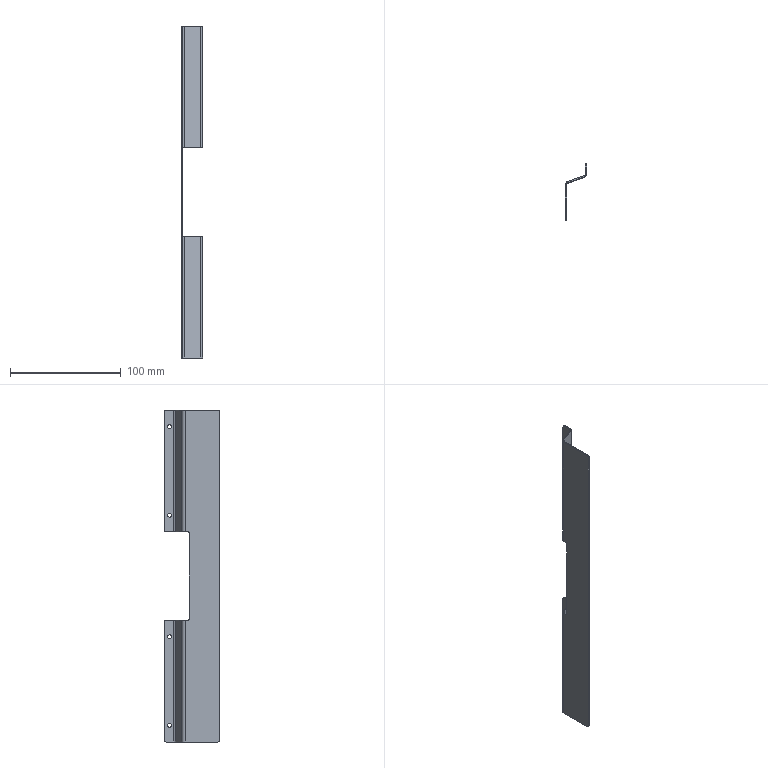Part | SolidWorks | features BaseBody 1 | 1 solid | 42 faces | box 19 x 50.551 x 300 mm | volume 15860 mm3 | cylinder 24 | plane 18 | commonest cylinder face diameters 4 x12 3.5 x8 6 x4
STEP:
#1=CARTESIAN_POINT('',(0.,6.,-53.25));
#2=VERTEX_POINT('',#1);
#3=CARTESIAN_POINT('',(0.,6.,-56.75));
#4=VERTEX_POINT('',#3);
#5=CARTESIAN_POINT('',(0.,6.,-55.));
#6=DIRECTION('',(1.,0.,0.));
#7=DIRECTION('',(0.,1.,0.));
#8=AXIS2_PLACEMENT_3D('',#5,#6,#7);
#9=CIRCLE('',#8,1.75);
#10=EDGE_CURVE('',#2,#4,#9,.T.);
#11=ORIENTED_EDGE('',*,*,#10,.T.);
#12=CARTESIAN_POINT('',(-1.,6.,-56.75));
#13=VERTEX_POINT('',#12);
#14=CARTESIAN_POINT('',(-1.,6.,-56.75));
#15=DIRECTION('',(-1.,0.,0.));
#16=VECTOR('',#15,1000.);
#17=LINE('',#14,#16);
#18=EDGE_CURVE('',#4,#13,#17,.T.);
#19=ORIENTED_EDGE('',*,*,#18,.T.);
#20=CARTESIAN_POINT('',(-1.,6.,-53.25));
#21=VERTEX_POINT('',#20);
#22=CARTESIAN_POINT('',(-1.,6.,-55.));
#23=DIRECTION('',(-1.,0.,0.));
#24=DIRECTION('',(0.,0.,1.));
#25=AXIS2_PLACEMENT_3D('',#22,#23,#24);
#26=CIRCLE('',#25,1.75);
#27=EDGE_CURVE('',#13,#21,#26,.T.);
#28=ORIENTED_EDGE('',*,*,#27,.T.);
#29=CARTESIAN_POINT('',(-1.,6.,-53.25));
#30=DIRECTION('',(-1.,0.,0.));
#31=VECTOR('',#30,1000.);
#32=LINE('',#29,#31);
#33=EDGE_CURVE('',#2,#21,#32,.T.);
#34=ORIENTED_EDGE('',*,*,#33,.F.);
#35=EDGE_LOOP('',(#11,#19,#28,#34));
#36=FACE_OUTER_BOUND('',#35,.T.);
#37=CARTESIAN_POINT('',(-1.,6.,-55.));
#38=DIRECTION('',(-1.,0.,0.));
#39=DIRECTION('',(0.,0.,1.));
#40=AXIS2_PLACEMENT_3D('',#37,#38,#39);
#41=CYLINDRICAL_SURFACE('',#40,1.75);
#42=ADVANCED_FACE('',(#36),#41,.F.);
#43=CARTESIAN_POINT('',(0.,6.,56.75));
#44=VERTEX_POINT('',#43);
#45=CARTESIAN_POINT('',(0.,6.,53.25));
#46=VERTEX_POINT('',#45);
#47=CARTESIAN_POINT('',(0.,6.,55.));
#48=DIRECTION('',(1.,0.,0.));
#49=DIRECTION('',(0.,1.,0.));
#50=AXIS2_PLACEMENT_3D('',#47,#48,#49);
#51=CIRCLE('',#50,1.75);
#52=EDGE_CURVE('',#44,#46,#51,.T.);
#53=ORIENTED_EDGE('',*,*,#52,.T.);
#54=CARTESIAN_POINT('',(-1.,6.,53.25));
#55=VERTEX_POINT('',#54);
#56=CARTESIAN_POINT('',(-1.,6.,53.25));
#57=DIRECTION('',(-1.,0.,0.));
#58=VECTOR('',#57,1000.);
#59=LINE('',#56,#58);
#60=EDGE_CURVE('',#46,#55,#59,.T.);
#61=ORIENTED_EDGE('',*,*,#60,.T.);
#62=CARTESIAN_POINT('',(-1.,6.,56.75));
#63=VERTEX_POINT('',#62);
#64=CARTESIAN_POINT('',(-1.,6.,55.));
#65=DIRECTION('',(-1.,0.,0.));
#66=DIRECTION('',(0.,0.,1.));
#67=AXIS2_PLACEMENT_3D('',#64,#65,#66);
#68=CIRCLE('',#67,1.75);
#69=EDGE_CURVE('',#55,#63,#68,.T.);
#70=ORIENTED_EDGE('',*,*,#69,.T.);
#71=CARTESIAN_POINT('',(-1.,6.,56.75));
#72=DIRECTION('',(-1.,0.,0.));
#73=VECTOR('',#72,1000.);
#74=LINE('',#71,#73);
#75=EDGE_CURVE('',#44,#63,#74,.T.);
#76=ORIENTED_EDGE('',*,*,#75,.F.);
#77=EDGE_LOOP('',(#53,#61,#70,#76));
#78=FACE_OUTER_BOUND('',#77,.T.);
#79=CARTESIAN_POINT('',(-1.,6.,55.));
#80=DIRECTION('',(-1.,0.,0.));
#81=DIRECTION('',(0.,0.,1.));
#82=AXIS2_PLACEMENT_3D('',#79,#80,#81);
#83=CYLINDRICAL_SURFACE('',#82,1.75);
#84=ADVANCED_FACE('',(#78),#83,.F.);
#85=CARTESIAN_POINT('',(0.,6.,-133.25));
#86=VERTEX_POINT('',#85);
#87=CARTESIAN_POINT('',(0.,6.,-136.75));
#88=VERTEX_POINT('',#87);
#89=CARTESIAN_POINT('',(0.,6.,-135.));
#90=DIRECTION('',(1.,0.,0.));
#91=DIRECTION('',(0.,1.,0.));
#92=AXIS2_PLACEMENT_3D('',#89,#90,#91);
#93=CIRCLE('',#92,1.75);
#94=EDGE_CURVE('',#86,#88,#93,.T.);
#95=ORIENTED_EDGE('',*,*,#94,.T.);
#96=CARTESIAN_POINT('',(-1.,6.,-136.75));
#97=VERTEX_POINT('',#96);
#98=CARTESIAN_POINT('',(-1.,6.,-136.75));
#99=DIRECTION('',(-1.,0.,0.));
#100=VECTOR('',#99,1000.);
#101=LINE('',#98,#100);
#102=EDGE_CURVE('',#88,#97,#101,.T.);
#103=ORIENTED_EDGE('',*,*,#102,.T.);
#104=CARTESIAN_POINT('',(-1.,6.,-133.25));
#105=VERTEX_POINT('',#104);
#106=CARTESIAN_POINT('',(-1.,6.,-135.));
#107=DIRECTION('',(-1.,0.,0.));
#108=DIRECTION('',(0.,0.,1.));
#109=AXIS2_PLACEMENT_3D('',#106,#107,#108);
#110=CIRCLE('',#109,1.75);
#111=EDGE_CURVE('',#97,#105,#110,.T.);
#112=ORIENTED_EDGE('',*,*,#111,.T.);
#113=CARTESIAN_POINT('',(-1.,6.,-133.25));
#114=DIRECTION('',(-1.,0.,0.));
#115=VECTOR('',#114,1000.);
#116=LINE('',#113,#115);
#117=EDGE_CURVE('',#86,#105,#116,.T.);
#118=ORIENTED_EDGE('',*,*,#117,.F.);
#119=EDGE_LOOP('',(#95,#103,#112,#118));
#120=FACE_OUTER_BOUND('',#119,.T.);
#121=CARTESIAN_POINT('',(-1.,6.,-135.));
#122=DIRECTION('',(-1.,0.,0.));
#123=DIRECTION('',(0.,0.,1.));
#124=AXIS2_PLACEMENT_3D('',#121,#122,#123);
#125=CYLINDRICAL_SURFACE('',#124,1.75);
#126=ADVANCED_FACE('',(#120),#125,.F.);
#127=CARTESIAN_POINT('',(0.,6.,136.75));
#128=VERTEX_POINT('',#127);
#129=CARTESIAN_POINT('',(0.,6.,133.25));
#130=VERTEX_POINT('',#129);
#131=CARTESIAN_POINT('',(0.,6.,135.));
#132=DIRECTION('',(1.,0.,0.));
#133=DIRECTION('',(0.,1.,0.));
#134=AXIS2_PLACEMENT_3D('',#131,#132,#133);
#135=CIRCLE('',#134,1.75);
#136=EDGE_CURVE('',#128,#130,#135,.T.);
#137=ORIENTED_EDGE('',*,*,#136,.T.);
#138=CARTESIAN_POINT('',(-1.,6.,133.25));
#139=VERTEX_POINT('',#138);
#140=CARTESIAN_POINT('',(-1.,6.,133.25));
#141=DIRECTION('',(-1.,0.,0.));
#142=VECTOR('',#141,1000.);
#143=LINE('',#140,#142);
#144=EDGE_CURVE('',#130,#139,#143,.T.);
#145=ORIENTED_EDGE('',*,*,#144,.T.);
#146=CARTESIAN_POINT('',(-1.,6.,136.75));
#147=VERTEX_POINT('',#146);
#148=CARTESIAN_POINT('',(-1.,6.,135.));
#149=DIRECTION('',(-1.,0.,0.));
#150=DIRECTION('',(0.,0.,1.));
#151=AXIS2_PLACEMENT_3D('',#148,#149,#150);
#152=CIRCLE('',#151,1.75);
#153=EDGE_CURVE('',#139,#147,#152,.T.);
#154=ORIENTED_EDGE('',*,*,#153,.T.);
#155=CARTESIAN_POINT('',(-1.,6.,136.75));
#156=DIRECTION('',(-1.,0.,0.));
#157=VECTOR('',#156,1000.);
#158=LINE('',#155,#157);
#159=EDGE_CURVE('',#128,#147,#158,.T.);
#160=ORIENTED_EDGE('',*,*,#159,.F.);
#161=EDGE_LOOP('',(#137,#145,#154,#160));
#162=FACE_OUTER_BOUND('',#161,.T.);
#163=CARTESIAN_POINT('',(-1.,6.,135.));
#164=DIRECTION('',(-1.,0.,0.));
#165=DIRECTION('',(0.,0.,1.));
#166=AXIS2_PLACEMENT_3D('',#163,#164,#165);
#167=CYLINDRICAL_SURFACE('',#166,1.75);
#168=ADVANCED_FACE('',(#162),#167,.F.);
#169=CARTESIAN_POINT('',(-1.,11.,-148.));
#170=VERTEX_POINT('',#169);
#171=CARTESIAN_POINT('',(-1.,9.,-150.));
#172=VERTEX_POINT('',#171);
#173=CARTESIAN_POINT('',(-1.,9.,-148.));
#174=DIRECTION('',(-1.,0.,0.));
#175=DIRECTION('',(0.,1.,0.));
#176=AXIS2_PLACEMENT_3D('',#173,#174,#175);
#177=CIRCLE('',#176,2.);
#178=EDGE_CURVE('',#170,#172,#177,.T.);
#179=ORIENTED_EDGE('',*,*,#178,.F.);
#180=CARTESIAN_POINT('',(0.,11.,-148.));
#181=VERTEX_POINT('',#180);
#182=CARTESIAN_POINT('',(-1.,11.,-148.));
#183=DIRECTION('',(-1.,0.,0.));
#184=VECTOR('',#183,1000.);
#185=LINE('',#182,#184);
#186=EDGE_CURVE('',#181,#170,#185,.T.);
#187=ORIENTED_EDGE('',*,*,#186,.F.);
#188=CARTESIAN_POINT('',(0.,9.,-150.));
#189=VERTEX_POINT('',#188);
#190=CARTESIAN_POINT('',(0.,9.,-148.));
#191=DIRECTION('',(1.,0.,0.));
#192=DIRECTION('',(0.,1.,0.));
#193=AXIS2_PLACEMENT_3D('',#190,#191,#192);
#194=CIRCLE('',#193,2.);
#195=EDGE_CURVE('',#189,#181,#194,.T.);
#196=ORIENTED_EDGE('',*,*,#195,.F.);
#197=CARTESIAN_POINT('',(-2.316,9.,-150.));
#198=DIRECTION('',(1.,0.,0.));
#199=VECTOR('',#198,1000.);
#200=LINE('',#197,#199);
#201=EDGE_CURVE('',#172,#189,#200,.T.);
#202=ORIENTED_EDGE('',*,*,#201,.F.);
#203=EDGE_LOOP('',(#179,#187,#196,#202));
#204=FACE_OUTER_BOUND('',#203,.T.);
#205=CARTESIAN_POINT('',(-2.316,9.,-148.));
#206=DIRECTION('',(1.,0.,0.));
#207=DIRECTION('',(0.,0.,-1.));
#208=AXIS2_PLACEMENT_3D('',#205,#206,#207);
#209=CYLINDRICAL_SURFACE('',#208,2.);
#210=ADVANCED_FACE('',(#204),#209,.T.);
#211=CARTESIAN_POINT('',(0.,11.,-42.));
#212=VERTEX_POINT('',#211);
#213=CARTESIAN_POINT('',(0.,9.,-40.));
#214=VERTEX_POINT('',#213);
#215=CARTESIAN_POINT('',(0.,9.,-42.));
#216=DIRECTION('',(1.,0.,0.));
#217=DIRECTION('',(0.,1.,0.));
#218=AXIS2_PLACEMENT_3D('',#215,#216,#217);
#219=CIRCLE('',#218,2.);
#220=EDGE_CURVE('',#212,#214,#219,.T.);
#221=ORIENTED_EDGE('',*,*,#220,.F.);
#222=CARTESIAN_POINT('',(-1.,11.,-42.));
#223=VERTEX_POINT('',#222);
#224=CARTESIAN_POINT('',(0.,11.,-42.));
#225=DIRECTION('',(1.,0.,0.));
#226=VECTOR('',#225,1000.);
#227=LINE('',#224,#226);
#228=EDGE_CURVE('',#223,#212,#227,.T.);
#229=ORIENTED_EDGE('',*,*,#228,.F.);
#230=CARTESIAN_POINT('',(-1.,9.,-40.));
#231=VERTEX_POINT('',#230);
#232=CARTESIAN_POINT('',(-1.,9.,-42.));
#233=DIRECTION('',(-1.,0.,0.));
#234=DIRECTION('',(0.,1.,0.));
#235=AXIS2_PLACEMENT_3D('',#232,#233,#234);
#236=CIRCLE('',#235,2.);
#237=EDGE_CURVE('',#231,#223,#236,.T.);
#238=ORIENTED_EDGE('',*,*,#237,.F.);
#239=CARTESIAN_POINT('',(-1.,9.,-40.));
#240=DIRECTION('',(-1.,0.,0.));
#241=VECTOR('',#240,1000.);
#242=LINE('',#239,#241);
#243=EDGE_CURVE('',#214,#231,#242,.T.);
#244=ORIENTED_EDGE('',*,*,#243,.F.);
#245=EDGE_LOOP('',(#221,#229,#238,#244));
#246=FACE_OUTER_BOUND('',#245,.T.);
#247=CARTESIAN_POINT('',(0.,9.,-42.));
#248=DIRECTION('',(1.,0.,0.));
#249=DIRECTION('',(0.,0.,-1.));
#250=AXIS2_PLACEMENT_3D('',#247,#248,#249);
#251=CYLINDRICAL_SURFACE('',#250,2.);
#252=ADVANCED_FACE('',(#246),#251,.T.);
#253=CARTESIAN_POINT('',(-18.,-10.,-40.));
#254=VERTEX_POINT('',#253);
#255=CARTESIAN_POINT('',(-18.,-12.,-38.));
#256=VERTEX_POINT('',#255);
#257=CARTESIAN_POINT('',(-18.,-10.,-38.));
#258=DIRECTION('',(-1.,0.,0.));
#259=DIRECTION('',(0.,1.,0.));
#260=AXIS2_PLACEMENT_3D('',#257,#258,#259);
#261=CIRCLE('',#260,2.);
#262=EDGE_CURVE('',#254,#256,#261,.T.);
#263=ORIENTED_EDGE('',*,*,#262,.F.);
#264=CARTESIAN_POINT('',(-19.,-10.,-40.));
#265=VERTEX_POINT('',#264);
#266=CARTESIAN_POINT('',(-18.,-10.,-40.));
#267=DIRECTION('',(1.,0.,0.));
#268=VECTOR('',#267,1000.);
#269=LINE('',#266,#268);
#270=EDGE_CURVE('',#265,#254,#269,.T.);
#271=ORIENTED_EDGE('',*,*,#270,.F.);
#272=CARTESIAN_POINT('',(-19.,-12.,-38.));
#273=VERTEX_POINT('',#272);
#274=CARTESIAN_POINT('',(-19.,-10.,-38.));
#275=DIRECTION('',(1.,0.,0.));
#276=DIRECTION('',(0.,1.,0.));
#277=AXIS2_PLACEMENT_3D('',#274,#275,#276);
#278=CIRCLE('',#277,2.);
#279=EDGE_CURVE('',#273,#265,#278,.T.);
#280=ORIENTED_EDGE('',*,*,#279,.F.);
#281=CARTESIAN_POINT('',(-19.,-12.,-38.));
#282=DIRECTION('',(-1.,0.,0.));
#283=VECTOR('',#282,1000.);
#284=LINE('',#281,#283);
#285=EDGE_CURVE('',#256,#273,#284,.T.);
#286=ORIENTED_EDGE('',*,*,#285,.F.);
#287=EDGE_LOOP('',(#263,#271,#280,#286));
#288=FACE_OUTER_BOUND('',#287,.T.);
#289=CARTESIAN_POINT('',(0.,-10.,-38.));
#290=DIRECTION('',(1.,0.,0.));
#291=DIRECTION('',(0.,1.,0.));
#292=AXIS2_PLACEMENT_3D('',#289,#290,#291);
#293=CYLINDRICAL_SURFACE('',#292,2.);
#294=ADVANCED_FACE('',(#288),#293,.F.);
#295=CARTESIAN_POINT('',(-18.,-12.,38.));
#296=VERTEX_POINT('',#295);
#297=CARTESIAN_POINT('',(-18.,-10.,40.));
#298=VERTEX_POINT('',#297);
#299=CARTESIAN_POINT('',(-18.,-10.,38.));
#300=DIRECTION('',(-1.,0.,0.));
#301=DIRECTION('',(0.,1.,0.));
#302=AXIS2_PLACEMENT_3D('',#299,#300,#301);
#303=CIRCLE('',#302,2.);
#304=EDGE_CURVE('',#296,#298,#303,.T.);
#305=ORIENTED_EDGE('',*,*,#304,.F.);
#306=CARTESIAN_POINT('',(-19.,-12.,38.));
#307=VERTEX_POINT('',#306);
#308=CARTESIAN_POINT('',(-18.,-12.,38.));
#309=DIRECTION('',(1.,0.,0.));
#310=VECTOR('',#309,1000.);
#311=LINE('',#308,#310);
#312=EDGE_CURVE('',#307,#296,#311,.T.);
#313=ORIENTED_EDGE('',*,*,#312,.F.);
#314=CARTESIAN_POINT('',(-19.,-10.,40.));
#315=VERTEX_POINT('',#314);
#316=CARTESIAN_POINT('',(-19.,-10.,38.));
#317=DIRECTION('',(1.,0.,0.));
#318=DIRECTION('',(0.,1.,0.));
#319=AXIS2_PLACEMENT_3D('',#316,#317,#318);
#320=CIRCLE('',#319,2.);
#321=EDGE_CURVE('',#315,#307,#320,.T.);
#322=ORIENTED_EDGE('',*,*,#321,.F.);
#323=CARTESIAN_POINT('',(-19.,-10.,40.));
#324=DIRECTION('',(-1.,0.,0.));
#325=VECTOR('',#324,1000.);
#326=LINE('',#323,#325);
#327=EDGE_CURVE('',#298,#315,#326,.T.);
#328=ORIENTED_EDGE('',*,*,#327,.F.);
#329=EDGE_LOOP('',(#305,#313,#322,#328));
#330=FACE_OUTER_BOUND('',#329,.T.);
#331=CARTESIAN_POINT('',(0.,-10.,38.));
#332=DIRECTION('',(1.,0.,0.));
#333=DIRECTION('',(0.,1.,0.));
#334=AXIS2_PLACEMENT_3D('',#331,#332,#333);
#335=CYLINDRICAL_SURFACE('',#334,2.);
#336=ADVANCED_FACE('',(#330),#335,.F.);
#337=CARTESIAN_POINT('',(0.,9.,40.));
#338=VERTEX_POINT('',#337);
#339=CARTESIAN_POINT('',(0.,11.,42.));
#340=VERTEX_POINT('',#339);
#341=CARTESIAN_POINT('',(0.,9.,42.));
#342=DIRECTION('',(1.,0.,0.));
#343=DIRECTION('',(0.,1.,0.));
#344=AXIS2_PLACEMENT_3D('',#341,#342,#343);
#345=CIRCLE('',#344,2.);
#346=EDGE_CURVE('',#338,#340,#345,.T.);
#347=ORIENTED_EDGE('',*,*,#346,.F.);
#348=CARTESIAN_POINT('',(-1.,9.,40.));
#349=VERTEX_POINT('',#348);
#350=CARTESIAN_POINT('',(0.,9.,40.));
#351=DIRECTION('',(1.,0.,0.));
#352=VECTOR('',#351,1000.);
#353=LINE('',#350,#352);
#354=EDGE_CURVE('',#349,#338,#353,.T.);
#355=ORIENTED_EDGE('',*,*,#354,.F.);
#356=CARTESIAN_POINT('',(-1.,11.,42.));
#357=VERTEX_POINT('',#356);
#358=CARTESIAN_POINT('',(-1.,9.,42.));
#359=DIRECTION('',(-1.,0.,0.));
#360=DIRECTION('',(0.,1.,0.));
#361=AXIS2_PLACEMENT_3D('',#358,#359,#360);
#362=CIRCLE('',#361,2.);
#363=EDGE_CURVE('',#357,#349,#362,.T.);
#364=ORIENTED_EDGE('',*,*,#363,.F.);
#365=CARTESIAN_POINT('',(-1.,11.,42.));
#366=DIRECTION('',(-1.,0.,0.));
#367=VECTOR('',#366,1000.);
#368=LINE('',#365,#367);
#369=EDGE_CURVE('',#340,#357,#368,.T.);
#370=ORIENTED_EDGE('',*,*,#369,.F.);
#371=EDGE_LOOP('',(#347,#355,#364,#370));
#372=FACE_OUTER_BOUND('',#371,.T.);
#373=CARTESIAN_POINT('',(-1.,9.,42.));
#374=DIRECTION('',(1.,0.,0.));
#375=DIRECTION('',(0.,0.,-1.));
#376=AXIS2_PLACEMENT_3D('',#373,#374,#375);
#377=CYLINDRICAL_SURFACE('',#376,2.);
#378=ADVANCED_FACE('',(#372),#377,.T.);
#379=CARTESIAN_POINT('',(-1.,9.,150.));
#380=VERTEX_POINT('',#379);
#381=CARTESIAN_POINT('',(-1.,11.,148.));
#382=VERTEX_POINT('',#381);
#383=CARTESIAN_POINT('',(-1.,9.,148.));
#384=DIRECTION('',(-1.,0.,0.));
#385=DIRECTION('',(0.,1.,0.));
#386=AXIS2_PLACEMENT_3D('',#383,#384,#385);
#387=CIRCLE('',#386,2.);
#388=EDGE_CURVE('',#380,#382,#387,.T.);
#389=ORIENTED_EDGE('',*,*,#388,.F.);
#390=CARTESIAN_POINT('',(0.,9.,150.));
#391=VERTEX_POINT('',#390);
#392=CARTESIAN_POINT('',(-1.,9.,150.));
#393=DIRECTION('',(-1.,0.,0.));
#394=VECTOR('',#393,1000.);
#395=LINE('',#392,#394);
#396=EDGE_CURVE('',#391,#380,#395,.T.);
#397=ORIENTED_EDGE('',*,*,#396,.F.);
#398=CARTESIAN_POINT('',(0.,11.,148.));
#399=VERTEX_POINT('',#398);
#400=CARTESIAN_POINT('',(0.,9.,148.));
#401=DIRECTION('',(1.,0.,0.));
#402=DIRECTION('',(0.,1.,0.));
#403=AXIS2_PLACEMENT_3D('',#400,#401,#402);
#404=CIRCLE('',#403,2.);
#405=EDGE_CURVE('',#399,#391,#404,.T.);
#406=ORIENTED_EDGE('',*,*,#405,.F.);
#407=CARTESIAN_POINT('',(0.,11.,148.));
#408=DIRECTION('',(1.,0.,0.));
#409=VECTOR('',#408,1000.);
#410=LINE('',#407,#409);
#411=EDGE_CURVE('',#382,#399,#410,.T.);
#412=ORIENTED_EDGE('',*,*,#411,.F.);
#413=EDGE_LOOP('',(#389,#397,#406,#412));
#414=FACE_OUTER_BOUND('',#413,.T.);
#415=CARTESIAN_POINT('',(-1.,9.,148.));
#416=DIRECTION('',(-1.,0.,0.));
#417=DIRECTION('',(0.,0.,1.));
#418=AXIS2_PLACEMENT_3D('',#415,#416,#417);
#419=CYLINDRICAL_SURFACE('',#418,2.);
#420=ADVANCED_FACE('',(#414),#419,.T.);
#421=CARTESIAN_POINT('',(-18.,-37.551,150.));
#422=VERTEX_POINT('',#421);
#423=CARTESIAN_POINT('',(-18.,-39.551,148.));
#424=VERTEX_POINT('',#423);
#425=CARTESIAN_POINT('',(-18.,-37.551,148.));
#426=DIRECTION('',(1.,0.,0.));
#427=DIRECTION('',(0.,1.,0.));
#428=AXIS2_PLACEMENT_3D('',#425,#426,#427);
#429=CIRCLE('',#428,2.);
#430=EDGE_CURVE('',#422,#424,#429,.T.);
#431=ORIENTED_EDGE('',*,*,#430,.F.);
#432=CARTESIAN_POINT('',(-19.,-37.551,150.));
#433=VERTEX_POINT('',#432);
#434=CARTESIAN_POINT('',(-17.026,-37.551,150.));
#435=DIRECTION('',(1.,0.,0.));
#436=VECTOR('',#435,1000.);
#437=LINE('',#434,#436);
#438=EDGE_CURVE('',#433,#422,#437,.T.);
#439=ORIENTED_EDGE('',*,*,#438,.F.);
#440=CARTESIAN_POINT('',(-19.,-39.551,148.));
#441=VERTEX_POINT('',#440);
#442=CARTESIAN_POINT('',(-19.,-37.551,148.));
#443=DIRECTION('',(-1.,0.,0.));
#444=DIRECTION('',(0.,1.,0.));
#445=AXIS2_PLACEMENT_3D('',#442,#443,#444);
#446=CIRCLE('',#445,2.);
#447=EDGE_CURVE('',#441,#433,#446,.T.);
#448=ORIENTED_EDGE('',*,*,#447,.F.);
#449=CARTESIAN_POINT('',(-18.,-39.551,148.));
#450=DIRECTION('',(-1.,0.,0.));
#451=VECTOR('',#450,1000.);
#452=LINE('',#449,#451);
#453=EDGE_CURVE('',#424,#441,#452,.T.);
#454=ORIENTED_EDGE('',*,*,#453,.F.);
#455=EDGE_LOOP('',(#431,#439,#448,#454));
#456=FACE_OUTER_BOUND('',#455,.T.);
#457=CARTESIAN_POINT('',(-18.,-37.551,148.));
#458=DIRECTION('',(-1.,0.,0.));
#459=DIRECTION('',(0.,0.,1.));
#460=AXIS2_PLACEMENT_3D('',#457,#458,#459);
#461=CYLINDRICAL_SURFACE('',#460,2.);
#462=ADVANCED_FACE('',(#456),#461,.T.);
#463=CARTESIAN_POINT('',(-18.,-39.551,-148.));
#464=VERTEX_POINT('',#463);
#465=CARTESIAN_POINT('',(-18.,-37.551,-150.));
#466=VERTEX_POINT('',#465);
#467=CARTESIAN_POINT('',(-18.,-37.551,-148.));
#468=DIRECTION('',(1.,0.,0.));
#469=DIRECTION('',(0.,1.,0.));
#470=AXIS2_PLACEMENT_3D('',#467,#468,#469);
#471=CIRCLE('',#470,2.);
#472=EDGE_CURVE('',#464,#466,#471,.T.);
#473=ORIENTED_EDGE('',*,*,#472,.F.);
#474=CARTESIAN_POINT('',(-19.,-39.551,-148.));
#475=VERTEX_POINT('',#474);
#476=CARTESIAN_POINT('',(-18.,-39.551,-148.));
#477=DIRECTION('',(1.,0.,0.));
#478=VECTOR('',#477,1000.);
#479=LINE('',#476,#478);
#480=EDGE_CURVE('',#475,#464,#479,.T.);
#481=ORIENTED_EDGE('',*,*,#480,.F.);
#482=CARTESIAN_POINT('',(-19.,-37.551,-150.));
#483=VERTEX_POINT('',#482);
#484=CARTESIAN_POINT('',(-19.,-37.551,-148.));
#485=DIRECTION('',(-1.,0.,0.));
#486=DIRECTION('',(0.,1.,0.));
#487=AXIS2_PLACEMENT_3D('',#484,#485,#486);
#488=CIRCLE('',#487,2.);
#489=EDGE_CURVE('',#483,#475,#488,.T.);
#490=ORIENTED_EDGE('',*,*,#489,.F.);
#491=CARTESIAN_POINT('',(-16.,-37.551,-150.));
#492=DIRECTION('',(-1.,0.,0.));
#493=VECTOR('',#492,1000.);
#494=LINE('',#491,#493);
#495=EDGE_CURVE('',#466,#483,#494,.T.);
#496=ORIENTED_EDGE('',*,*,#495,.F.);
#497=EDGE_LOOP('',(#473,#481,#490,#496));
#498=FACE_OUTER_BOUND('',#497,.T.);
#499=CARTESIAN_POINT('',(-16.,-37.551,-148.));
#500=DIRECTION('',(-1.,0.,0.));
#501=DIRECTION('',(0.,0.,1.));
#502=AXIS2_PLACEMENT_3D('',#499,#500,#501);
#503=CYLINDRICAL_SURFACE('',#502,2.);
#504=ADVANCED_FACE('',(#498),#503,.T.);
#505=CARTESIAN_POINT('',(-19.,-12.,-40.));
#506=DIRECTION('',(0.,0.,1.));
#507=VECTOR('',#506,1000.);
#508=LINE('',#505,#507);
#509=EDGE_CURVE('',#273,#307,#508,.T.);
#510=ORIENTED_EDGE('',*,*,#509,.T.);
#511=ORIENTED_EDGE('',*,*,#312,.T.);
#512=CARTESIAN_POINT('',(-18.,-12.,150.));
#513=DIRECTION('',(0.,0.,-1.));
#514=VECTOR('',#513,1000.);
#515=LINE('',#512,#514);
#516=EDGE_CURVE('',#296,#256,#515,.T.);
#517=ORIENTED_EDGE('',*,*,#516,.T.);
#518=ORIENTED_EDGE('',*,*,#285,.T.);
#519=EDGE_LOOP('',(#510,#511,#517,#518));
#520=FACE_OUTER_BOUND('',#519,.T.);
#521=CARTESIAN_POINT('',(0.,-12.,-40.));
#522=DIRECTION('',(0.,-1.,0.));
#523=DIRECTION('',(0.,0.,-1.));
#524=AXIS2_PLACEMENT_3D('',#521,#522,#523);
#525=PLANE('',#524);
#526=ADVANCED_FACE('',(#520),#525,.F.);
#527=CARTESIAN_POINT('',(-17.026,-5.133,150.));
#528=VERTEX_POINT('',#527);
#529=CARTESIAN_POINT('',(-17.026,-5.133,40.));
#530=VERTEX_POINT('',#529);
#531=CARTESIAN_POINT('',(-17.026,-5.133,150.));
#532=DIRECTION('',(0.,0.,-1.));
#533=VECTOR('',#532,1000.);
#534=LINE('',#531,#533);
#535=EDGE_CURVE('',#528,#530,#534,.T.);
#536=ORIENTED_EDGE('',*,*,#535,.T.);
#537=CARTESIAN_POINT('',(-19.,-7.952,40.));
#538=VERTEX_POINT('',#537);
#539=CARTESIAN_POINT('',(-16.,-7.952,40.));
#540=DIRECTION('',(0.,0.,1.));
#541=DIRECTION('',(0.,-1.,0.));
#542=AXIS2_PLACEMENT_3D('',#539,#540,#541);
#543=CIRCLE('',#542,3.);
#544=EDGE_CURVE('',#530,#538,#543,.T.);
#545=ORIENTED_EDGE('',*,*,#544,.T.);
#546=CARTESIAN_POINT('',(-19.,-7.952,150.));
#547=VERTEX_POINT('',#546);
#548=CARTESIAN_POINT('',(-19.,-7.952,150.));
#549=DIRECTION('',(0.,0.,-1.));
#550=VECTOR('',#549,1000.);
#551=LINE('',#548,#550);
#552=EDGE_CURVE('',#547,#538,#551,.T.);
#553=ORIENTED_EDGE('',*,*,#552,.F.);
#554=CARTESIAN_POINT('',(-16.,-7.952,150.));
#555=DIRECTION('',(0.,0.,1.));
#556=DIRECTION('',(1.,0.,0.));
#557=AXIS2_PLACEMENT_3D('',#554,#555,#556);
#558=CIRCLE('',#557,3.);
#559=EDGE_CURVE('',#528,#547,#558,.T.);
#560=ORIENTED_EDGE('',*,*,#559,.F.);
#561=EDGE_LOOP('',(#536,#545,#553,#560));
#562=FACE_OUTER_BOUND('',#561,.T.);
#563=CARTESIAN_POINT('',(-16.,-7.952,150.));
#564=DIRECTION('',(0.,0.,-1.));
#565=DIRECTION('',(-1.,0.,0.));
#566=AXIS2_PLACEMENT_3D('',#563,#564,#565);
#567=CYLINDRICAL_SURFACE('',#566,3.);
#568=ADVANCED_FACE('',(#562),#567,.T.);
#569=CARTESIAN_POINT('',(-2.316,0.2212,150.));
#570=VERTEX_POINT('',#569);
#571=CARTESIAN_POINT('',(-2.316,0.2212,40.));
#572=VERTEX_POINT('',#571);
#573=CARTESIAN_POINT('',(-2.316,0.2212,150.));
#574=DIRECTION('',(0.,0.,-1.));
#575=VECTOR('',#574,1000.);
#576=LINE('',#573,#575);
#577=EDGE_CURVE('',#570,#572,#576,.T.);
#578=ORIENTED_EDGE('',*,*,#577,.T.);
#579=CARTESIAN_POINT('',(-0.342,0.9397,40.));
#580=DIRECTION('',(-0.9397,-0.342,0.));
#581=VECTOR('',#580,1000.);
#582=LINE('',#579,#581);
#583=EDGE_CURVE('',#572,#530,#582,.T.);
#584=ORIENTED_EDGE('',*,*,#583,.T.);
#585=ORIENTED_EDGE('',*,*,#535,.F.);
#586=CARTESIAN_POINT('',(-0.342,0.9397,150.));
#587=DIRECTION('',(-0.9397,-0.342,0.));
#588=VECTOR('',#587,1000.);
#589=LINE('',#586,#588);
#590=EDGE_CURVE('',#570,#528,#589,.T.);
#591=ORIENTED_EDGE('',*,*,#590,.F.);
#592=EDGE_LOOP('',(#578,#584,#585,#591));
#593=FACE_OUTER_BOUND('',#592,.T.);
#594=CARTESIAN_POINT('',(-0.342,0.9397,150.));
#595=DIRECTION('',(0.342,-0.9397,0.));
#596=DIRECTION('',(0.,0.,-1.));
#597=AXIS2_PLACEMENT_3D('',#594,#595,#596);
#598=PLANE('',#597);
#599=ADVANCED_FACE('',(#593),#598,.F.);
#600=CARTESIAN_POINT('',(-1.,2.101,150.));
#601=VERTEX_POINT('',#600);
#602=CARTESIAN_POINT('',(-1.,2.101,40.));
#603=VERTEX_POINT('',#602);
#604=CARTESIAN_POINT('',(-1.,2.101,150.));
#605=DIRECTION('',(0.,0.,-1.));
#606=VECTOR('',#605,1000.);
#607=LINE('',#604,#606);
#608=EDGE_CURVE('',#601,#603,#607,.T.);
#609=ORIENTED_EDGE('',*,*,#608,.T.);
#610=CARTESIAN_POINT('',(-3.,2.101,40.));
#611=DIRECTION('',(0.,0.,-1.));
#612=DIRECTION('',(0.,-1.,0.));
#613=AXIS2_PLACEMENT_3D('',#610,#611,#612);
#614=CIRCLE('',#613,2.);
#615=EDGE_CURVE('',#603,#572,#614,.T.);
#616=ORIENTED_EDGE('',*,*,#615,.T.);
#617=ORIENTED_EDGE('',*,*,#577,.F.);
#618=CARTESIAN_POINT('',(-3.,2.101,150.));
#619=DIRECTION('',(0.,0.,-1.));
#620=DIRECTION('',(1.,0.,0.));
#621=AXIS2_PLACEMENT_3D('',#618,#619,#620);
#622=CIRCLE('',#621,2.);
#623=EDGE_CURVE('',#601,#570,#622,.T.);
#624=ORIENTED_EDGE('',*,*,#623,.F.);
#625=EDGE_LOOP('',(#609,#616,#617,#624));
#626=FACE_OUTER_BOUND('',#625,.T.);
#627=CARTESIAN_POINT('',(-3.,2.101,150.));
#628=DIRECTION('',(0.,0.,-1.));
#629=DIRECTION('',(-1.,0.,0.));
#630=AXIS2_PLACEMENT_3D('',#627,#628,#629);
#631=CYLINDRICAL_SURFACE('',#630,2.);
#632=ADVANCED_FACE('',(#626),#631,.F.);
#633=CARTESIAN_POINT('',(-1.,11.,150.));
#634=DIRECTION('',(0.,0.,-1.));
#635=VECTOR('',#634,1000.);
#636=LINE('',#633,#635);
#637=EDGE_CURVE('',#382,#357,#636,.T.);
#638=ORIENTED_EDGE('',*,*,#637,.F.);
#639=ORIENTED_EDGE('',*,*,#411,.T.);
#640=CARTESIAN_POINT('',(0.,11.,150.));
#641=DIRECTION('',(0.,0.,-1.));
#642=VECTOR('',#641,1000.);
#643=LINE('',#640,#642);
#644=EDGE_CURVE('',#399,#340,#643,.T.);
#645=ORIENTED_EDGE('',*,*,#644,.T.);
#646=ORIENTED_EDGE('',*,*,#369,.T.);
#647=EDGE_LOOP('',(#638,#639,#645,#646));
#648=FACE_OUTER_BOUND('',#647,.T.);
#649=CARTESIAN_POINT('',(-1.,11.,150.));
#650=DIRECTION('',(0.,1.,0.));
#651=DIRECTION('',(1.,0.,0.));
#652=AXIS2_PLACEMENT_3D('',#649,#650,#651);
#653=PLANE('',#652);
#654=ADVANCED_FACE('',(#648),#653,.T.);
#655=ORIENTED_EDGE('',*,*,#136,.F.);
#656=CARTESIAN_POINT('',(0.,6.,135.));
#657=DIRECTION('',(1.,0.,0.));
#658=DIRECTION('',(0.,1.,0.));
#659=AXIS2_PLACEMENT_3D('',#656,#657,#658);
#660=CIRCLE('',#659,1.75);
#661=EDGE_CURVE('',#130,#128,#660,.T.);
#662=ORIENTED_EDGE('',*,*,#661,.F.);
#663=EDGE_LOOP('',(#655,#662));
#664=FACE_BOUND('',#663,.T.);
#665=ORIENTED_EDGE('',*,*,#52,.F.);
#666=CARTESIAN_POINT('',(0.,6.,55.));
#667=DIRECTION('',(1.,0.,0.));
#668=DIRECTION('',(0.,1.,0.));
#669=AXIS2_PLACEMENT_3D('',#666,#667,#668);
#670=CIRCLE('',#669,1.75);
#671=EDGE_CURVE('',#46,#44,#670,.T.);
#672=ORIENTED_EDGE('',*,*,#671,.F.);
#673=EDGE_LOOP('',(#665,#672));
#674=FACE_BOUND('',#673,.T.);
#675=ORIENTED_EDGE('',*,*,#644,.F.);
#676=ORIENTED_EDGE('',*,*,#405,.T.);
#677=CARTESIAN_POINT('',(0.,2.101,150.));
#678=VERTEX_POINT('',#677);
#679=CARTESIAN_POINT('',(0.,11.,150.));
#680=DIRECTION('',(0.,-1.,0.));
#681=VECTOR('',#680,1000.);
#682=LINE('',#679,#681);
#683=EDGE_CURVE('',#391,#678,#682,.T.);
#684=ORIENTED_EDGE('',*,*,#683,.T.);
#685=CARTESIAN_POINT('',(0.,2.101,40.));
#686=VERTEX_POINT('',#685);
#687=CARTESIAN_POINT('',(0.,2.101,150.));
#688=DIRECTION('',(0.,0.,-1.));
#689=VECTOR('',#688,1000.);
#690=LINE('',#687,#689);
#691=EDGE_CURVE('',#678,#686,#690,.T.);
#692=ORIENTED_EDGE('',*,*,#691,.T.);
#693=CARTESIAN_POINT('',(0.,11.,40.));
#694=DIRECTION('',(0.,1.,0.));
#695=VECTOR('',#694,1000.);
#696=LINE('',#693,#695);
#697=EDGE_CURVE('',#686,#338,#696,.T.);
#698=ORIENTED_EDGE('',*,*,#697,.T.);
#699=ORIENTED_EDGE('',*,*,#346,.T.);
#700=EDGE_LOOP('',(#675,#676,#684,#692,#698,#699));
#701=FACE_OUTER_BOUND('',#700,.T.);
#702=CARTESIAN_POINT('',(0.,11.,150.));
#703=DIRECTION('',(1.,0.,0.));
#704=DIRECTION('',(0.,-1.,0.));
#705=AXIS2_PLACEMENT_3D('',#702,#703,#704);
#706=PLANE('',#705);
#707=ADVANCED_FACE('',(#664,#674,#701),#706,.T.);
#708=CARTESIAN_POINT('',(-1.974,-0.7185,40.));
#709=VERTEX_POINT('',#708);
#710=CARTESIAN_POINT('',(-3.,2.101,40.));
#711=DIRECTION('',(0.,0.,-1.));
#712=DIRECTION('',(0.,-1.,0.));
#713=AXIS2_PLACEMENT_3D('',#710,#711,#712);
#714=CIRCLE('',#713,3.);
#715=EDGE_CURVE('',#686,#709,#714,.T.);
#716=ORIENTED_EDGE('',*,*,#715,.F.);
#717=ORIENTED_EDGE('',*,*,#691,.F.);
#718=CARTESIAN_POINT('',(-1.974,-0.7185,150.));
#719=VERTEX_POINT('',#718);
#720=CARTESIAN_POINT('',(-3.,2.101,150.));
#721=DIRECTION('',(0.,0.,-1.));
#722=DIRECTION('',(1.,0.,0.));
#723=AXIS2_PLACEMENT_3D('',#720,#721,#722);
#724=CIRCLE('',#723,3.);
#725=EDGE_CURVE('',#678,#719,#724,.T.);
#726=ORIENTED_EDGE('',*,*,#725,.T.);
#727=CARTESIAN_POINT('',(-1.974,-0.7185,150.));
#728=DIRECTION('',(0.,0.,-1.));
#729=VECTOR('',#728,1000.);
#730=LINE('',#727,#729);
#731=EDGE_CURVE('',#719,#709,#730,.T.);
#732=ORIENTED_EDGE('',*,*,#731,.T.);
#733=EDGE_LOOP('',(#716,#717,#726,#732));
#734=FACE_OUTER_BOUND('',#733,.T.);
#735=CARTESIAN_POINT('',(-3.,2.101,150.));
#736=DIRECTION('',(0.,0.,-1.));
#737=DIRECTION('',(-1.,0.,0.));
#738=AXIS2_PLACEMENT_3D('',#735,#736,#737);
#739=CYLINDRICAL_SURFACE('',#738,3.);
#740=ADVANCED_FACE('',(#734),#739,.T.);
#741=CARTESIAN_POINT('',(-16.684,-6.072,40.));
#742=VERTEX_POINT('',#741);
#743=CARTESIAN_POINT('',(0.,0.,40.));
#744=DIRECTION('',(-0.9397,-0.342,0.));
#745=VECTOR('',#744,1000.);
#746=LINE('',#743,#745);
#747=EDGE_CURVE('',#709,#742,#746,.T.);
#748=ORIENTED_EDGE('',*,*,#747,.F.);
#749=ORIENTED_EDGE('',*,*,#731,.F.);
#750=CARTESIAN_POINT('',(-16.684,-6.072,150.));
#751=VERTEX_POINT('',#750);
#752=CARTESIAN_POINT('',(0.,0.,150.));
#753=DIRECTION('',(-0.9397,-0.342,0.));
#754=VECTOR('',#753,1000.);
#755=LINE('',#752,#754);
#756=EDGE_CURVE('',#719,#751,#755,.T.);
#757=ORIENTED_EDGE('',*,*,#756,.T.);
#758=CARTESIAN_POINT('',(-16.684,-6.072,150.));
#759=DIRECTION('',(0.,0.,-1.));
#760=VECTOR('',#759,1000.);
#761=LINE('',#758,#760);
#762=EDGE_CURVE('',#751,#742,#761,.T.);
#763=ORIENTED_EDGE('',*,*,#762,.T.);
#764=EDGE_LOOP('',(#748,#749,#757,#763));
#765=FACE_OUTER_BOUND('',#764,.T.);
#766=CARTESIAN_POINT('',(0.,0.,150.));
#767=DIRECTION('',(0.342,-0.9397,0.));
#768=DIRECTION('',(0.,0.,-1.));
#769=AXIS2_PLACEMENT_3D('',#766,#767,#768);
#770=PLANE('',#769);
#771=ADVANCED_FACE('',(#765),#770,.T.);
#772=CARTESIAN_POINT('',(-18.,-7.952,40.));
#773=VERTEX_POINT('',#772);
#774=CARTESIAN_POINT('',(-16.,-7.952,40.));
#775=DIRECTION('',(0.,0.,1.));
#776=DIRECTION('',(0.,-1.,0.));
#777=AXIS2_PLACEMENT_3D('',#774,#775,#776);
#778=CIRCLE('',#777,2.);
#779=EDGE_CURVE('',#742,#773,#778,.T.);
#780=ORIENTED_EDGE('',*,*,#779,.F.);
#781=ORIENTED_EDGE('',*,*,#762,.F.);
#782=CARTESIAN_POINT('',(-18.,-7.952,150.));
#783=VERTEX_POINT('',#782);
#784=CARTESIAN_POINT('',(-16.,-7.952,150.));
#785=DIRECTION('',(0.,0.,1.));
#786=DIRECTION('',(-1.,0.,0.));
#787=AXIS2_PLACEMENT_3D('',#784,#785,#786);
#788=CIRCLE('',#787,2.);
#789=EDGE_CURVE('',#751,#783,#788,.T.);
#790=ORIENTED_EDGE('',*,*,#789,.T.);
#791=CARTESIAN_POINT('',(-18.,-7.952,150.));
#792=DIRECTION('',(0.,0.,-1.));
#793=VECTOR('',#792,1000.);
#794=LINE('',#791,#793);
#795=EDGE_CURVE('',#783,#773,#794,.T.);
#796=ORIENTED_EDGE('',*,*,#795,.T.);
#797=EDGE_LOOP('',(#780,#781,#790,#796));
#798=FACE_OUTER_BOUND('',#797,.T.);
#799=CARTESIAN_POINT('',(-16.,-7.952,150.));
#800=DIRECTION('',(0.,0.,-1.));
#801=DIRECTION('',(-1.,0.,0.));
#802=AXIS2_PLACEMENT_3D('',#799,#800,#801);
#803=CYLINDRICAL_SURFACE('',#802,2.);
#804=ADVANCED_FACE('',(#798),#803,.F.);
#805=CARTESIAN_POINT('',(-18.,-39.551,150.));
#806=DIRECTION('',(0.,0.,-1.));
#807=VECTOR('',#806,1000.);
#808=LINE('',#805,#807);
#809=EDGE_CURVE('',#424,#464,#808,.T.);
#810=ORIENTED_EDGE('',*,*,#809,.T.);
#811=ORIENTED_EDGE('',*,*,#472,.T.);
#812=CARTESIAN_POINT('',(-18.,-7.952,-150.));
#813=VERTEX_POINT('',#812);
#814=CARTESIAN_POINT('',(-18.,-6.551,-150.));
#815=DIRECTION('',(0.,-1.,0.));
#816=VECTOR('',#815,1000.);
#817=LINE('',#814,#816);
#818=EDGE_CURVE('',#813,#466,#817,.T.);
#819=ORIENTED_EDGE('',*,*,#818,.F.);
#820=CARTESIAN_POINT('',(-18.,-7.952,-40.));
#821=VERTEX_POINT('',#820);
#822=CARTESIAN_POINT('',(-18.,-7.952,150.));
#823=DIRECTION('',(0.,0.,-1.));
#824=VECTOR('',#823,1000.);
#825=LINE('',#822,#824);
#826=EDGE_CURVE('',#821,#813,#825,.T.);
#827=ORIENTED_EDGE('',*,*,#826,.F.);
#828=CARTESIAN_POINT('',(-18.,-6.551,-40.));
#829=DIRECTION('',(0.,1.,0.));
#830=VECTOR('',#829,1000.);
#831=LINE('',#828,#830);
#832=EDGE_CURVE('',#254,#821,#831,.T.);
#833=ORIENTED_EDGE('',*,*,#832,.F.);
#834=ORIENTED_EDGE('',*,*,#262,.T.);
#835=ORIENTED_EDGE('',*,*,#516,.F.);
#836=ORIENTED_EDGE('',*,*,#304,.T.);
#837=CARTESIAN_POINT('',(-18.,-6.551,40.));
#838=DIRECTION('',(0.,-1.,0.));
#839=VECTOR('',#838,1000.);
#840=LINE('',#837,#839);
#841=EDGE_CURVE('',#773,#298,#840,.T.);
#842=ORIENTED_EDGE('',*,*,#841,.F.);
#843=ORIENTED_EDGE('',*,*,#795,.F.);
#844=CARTESIAN_POINT('',(-18.,-6.551,150.));
#845=DIRECTION('',(0.,-1.,0.));
#846=VECTOR('',#845,1000.);
#847=LINE('',#844,#846);
#848=EDGE_CURVE('',#783,#422,#847,.T.);
#849=ORIENTED_EDGE('',*,*,#848,.T.);
#850=ORIENTED_EDGE('',*,*,#430,.T.);
#851=EDGE_LOOP('',(#810,#811,#819,#827,#833,#834,#835,#836,#842,#843,#849,#850));
#852=FACE_OUTER_BOUND('',#851,.T.);
#853=CARTESIAN_POINT('',(-18.,-6.551,150.));
#854=DIRECTION('',(1.,0.,0.));
#855=DIRECTION('',(0.,1.,0.));
#856=AXIS2_PLACEMENT_3D('',#853,#854,#855);
#857=PLANE('',#856);
#858=ADVANCED_FACE('',(#852),#857,.T.);
#859=CARTESIAN_POINT('',(-19.,-39.551,150.));
#860=DIRECTION('',(0.,0.,-1.));
#861=VECTOR('',#860,1000.);
#862=LINE('',#859,#861);
#863=EDGE_CURVE('',#441,#475,#862,.T.);
#864=ORIENTED_EDGE('',*,*,#863,.T.);
#865=ORIENTED_EDGE('',*,*,#480,.T.);
#866=ORIENTED_EDGE('',*,*,#809,.F.);
#867=ORIENTED_EDGE('',*,*,#453,.T.);
#868=EDGE_LOOP('',(#864,#865,#866,#867));
#869=FACE_OUTER_BOUND('',#868,.T.);
#870=CARTESIAN_POINT('',(-18.,-39.551,150.));
#871=DIRECTION('',(0.,-1.,0.));
#872=DIRECTION('',(0.,0.,-1.));
#873=AXIS2_PLACEMENT_3D('',#870,#871,#872);
#874=PLANE('',#873);
#875=ADVANCED_FACE('',(#869),#874,.T.);
#876=CARTESIAN_POINT('',(-19.,-7.952,-150.));
#877=VERTEX_POINT('',#876);
#878=CARTESIAN_POINT('',(-19.,-6.551,-150.));
#879=DIRECTION('',(0.,-1.,0.));
#880=VECTOR('',#879,1000.);
#881=LINE('',#878,#880);
#882=EDGE_CURVE('',#877,#483,#881,.T.);
#883=ORIENTED_EDGE('',*,*,#882,.T.);
#884=ORIENTED_EDGE('',*,*,#489,.T.);
#885=ORIENTED_EDGE('',*,*,#863,.F.);
#886=ORIENTED_EDGE('',*,*,#447,.T.);
#887=CARTESIAN_POINT('',(-19.,-6.551,150.));
#888=DIRECTION('',(0.,-1.,0.));
#889=VECTOR('',#888,1000.);
#890=LINE('',#887,#889);
#891=EDGE_CURVE('',#547,#433,#890,.T.);
#892=ORIENTED_EDGE('',*,*,#891,.F.);
#893=ORIENTED_EDGE('',*,*,#552,.T.);
#894=CARTESIAN_POINT('',(-19.,11.,40.));
#895=DIRECTION('',(0.,1.,0.));
#896=VECTOR('',#895,1000.);
#897=LINE('',#894,#896);
#898=EDGE_CURVE('',#315,#538,#897,.T.);
#899=ORIENTED_EDGE('',*,*,#898,.F.);
#900=ORIENTED_EDGE('',*,*,#321,.T.);
#901=ORIENTED_EDGE('',*,*,#509,.F.);
#902=ORIENTED_EDGE('',*,*,#279,.T.);
#903=CARTESIAN_POINT('',(-19.,-7.952,-40.));
#904=VERTEX_POINT('',#903);
#905=CARTESIAN_POINT('',(-19.,11.,-40.));
#906=DIRECTION('',(0.,-1.,0.));
#907=VECTOR('',#906,1000.);
#908=LINE('',#905,#907);
#909=EDGE_CURVE('',#904,#265,#908,.T.);
#910=ORIENTED_EDGE('',*,*,#909,.F.);
#911=CARTESIAN_POINT('',(-19.,-7.952,150.));
#912=DIRECTION('',(0.,0.,-1.));
#913=VECTOR('',#912,1000.);
#914=LINE('',#911,#913);
#915=EDGE_CURVE('',#904,#877,#914,.T.);
#916=ORIENTED_EDGE('',*,*,#915,.T.);
#917=EDGE_LOOP('',(#883,#884,#885,#886,#892,#893,#899,#900,#901,#902,#910,#916));
#918=FACE_OUTER_BOUND('',#917,.T.);
#919=CARTESIAN_POINT('',(-19.,-6.551,150.));
#920=DIRECTION('',(1.,0.,0.));
#921=DIRECTION('',(0.,1.,0.));
#922=AXIS2_PLACEMENT_3D('',#919,#920,#921);
#923=PLANE('',#922);
#924=ADVANCED_FACE('',(#918),#923,.F.);
#925=CARTESIAN_POINT('',(-1.,2.101,-150.));
#926=VERTEX_POINT('',#925);
#927=CARTESIAN_POINT('',(-2.316,0.2212,-150.));
#928=VERTEX_POINT('',#927);
#929=CARTESIAN_POINT('',(-3.,2.101,-150.));
#930=DIRECTION('',(0.,0.,-1.));
#931=DIRECTION('',(1.,0.,0.));
#932=AXIS2_PLACEMENT_3D('',#929,#930,#931);
#933=CIRCLE('',#932,2.);
#934=EDGE_CURVE('',#926,#928,#933,.T.);
#935=ORIENTED_EDGE('',*,*,#934,.F.);
#936=CARTESIAN_POINT('',(-1.,11.,-150.));
#937=DIRECTION('',(0.,-1.,0.));
#938=VECTOR('',#937,1000.);
#939=LINE('',#936,#938);
#940=EDGE_CURVE('',#172,#926,#939,.T.);
#941=ORIENTED_EDGE('',*,*,#940,.F.);
#942=ORIENTED_EDGE('',*,*,#201,.T.);
#943=CARTESIAN_POINT('',(0.,2.101,-150.));
#944=VERTEX_POINT('',#943);
#945=CARTESIAN_POINT('',(0.,11.,-150.));
#946=DIRECTION('',(0.,-1.,0.));
#947=VECTOR('',#946,1000.);
#948=LINE('',#945,#947);
#949=EDGE_CURVE('',#189,#944,#948,.T.);
#950=ORIENTED_EDGE('',*,*,#949,.T.);
#951=CARTESIAN_POINT('',(-1.974,-0.7185,-150.));
#952=VERTEX_POINT('',#951);
#953=CARTESIAN_POINT('',(-3.,2.101,-150.));
#954=DIRECTION('',(0.,0.,-1.));
#955=DIRECTION('',(1.,0.,0.));
#956=AXIS2_PLACEMENT_3D('',#953,#954,#955);
#957=CIRCLE('',#956,3.);
#958=EDGE_CURVE('',#944,#952,#957,.T.);
#959=ORIENTED_EDGE('',*,*,#958,.T.);
#960=CARTESIAN_POINT('',(-16.684,-6.072,-150.));
#961=VERTEX_POINT('',#960);
#962=CARTESIAN_POINT('',(0.,0.,-150.));
#963=DIRECTION('',(-0.9397,-0.342,0.));
#964=VECTOR('',#963,1000.);
#965=LINE('',#962,#964);
#966=EDGE_CURVE('',#952,#961,#965,.T.);
#967=ORIENTED_EDGE('',*,*,#966,.T.);
#968=CARTESIAN_POINT('',(-16.,-7.952,-150.));
#969=DIRECTION('',(0.,0.,1.));
#970=DIRECTION('',(-1.,0.,0.));
#971=AXIS2_PLACEMENT_3D('',#968,#969,#970);
#972=CIRCLE('',#971,2.);
#973=EDGE_CURVE('',#961,#813,#972,.T.);
#974=ORIENTED_EDGE('',*,*,#973,.T.);
#975=ORIENTED_EDGE('',*,*,#818,.T.);
#976=ORIENTED_EDGE('',*,*,#495,.T.);
#977=ORIENTED_EDGE('',*,*,#882,.F.);
#978=CARTESIAN_POINT('',(-17.026,-5.133,-150.));
#979=VERTEX_POINT('',#978);
#980=CARTESIAN_POINT('',(-16.,-7.952,-150.));
#981=DIRECTION('',(0.,0.,1.));
#982=DIRECTION('',(1.,0.,0.));
#983=AXIS2_PLACEMENT_3D('',#980,#981,#982);
#984=CIRCLE('',#983,3.);
#985=EDGE_CURVE('',#979,#877,#984,.T.);
#986=ORIENTED_EDGE('',*,*,#985,.F.);
#987=CARTESIAN_POINT('',(-0.342,0.9397,-150.));
#988=DIRECTION('',(-0.9397,-0.342,0.));
#989=VECTOR('',#988,1000.);
#990=LINE('',#987,#989);
#991=EDGE_CURVE('',#928,#979,#990,.T.);
#992=ORIENTED_EDGE('',*,*,#991,.F.);
#993=EDGE_LOOP('',(#935,#941,#942,#950,#959,#967,#974,#975,#976,#977,#986,#992));
#994=FACE_OUTER_BOUND('',#993,.T.);
#995=CARTESIAN_POINT('',(0.,2.101,-150.));
#996=DIRECTION('',(0.,0.,-1.));
#997=DIRECTION('',(0.,-1.,0.));
#998=AXIS2_PLACEMENT_3D('',#995,#996,#997);
#999=PLANE('',#998);
#1000=ADVANCED_FACE('',(#994),#999,.T.);
#1001=ORIENTED_EDGE('',*,*,#623,.T.);
#1002=ORIENTED_EDGE('',*,*,#590,.T.);
#1003=ORIENTED_EDGE('',*,*,#559,.T.);
#1004=ORIENTED_EDGE('',*,*,#891,.T.);
#1005=ORIENTED_EDGE('',*,*,#438,.T.);
#1006=ORIENTED_EDGE('',*,*,#848,.F.);
#1007=ORIENTED_EDGE('',*,*,#789,.F.);
#1008=ORIENTED_EDGE('',*,*,#756,.F.);
#1009=ORIENTED_EDGE('',*,*,#725,.F.);
#1010=ORIENTED_EDGE('',*,*,#683,.F.);
#1011=ORIENTED_EDGE('',*,*,#396,.T.);
#1012=CARTESIAN_POINT('',(-1.,11.,150.));
#1013=DIRECTION('',(0.,-1.,0.));
#1014=VECTOR('',#1013,1000.);
#1015=LINE('',#1012,#1014);
#1016=EDGE_CURVE('',#380,#601,#1015,.T.);
#1017=ORIENTED_EDGE('',*,*,#1016,.T.);
#1018=EDGE_LOOP('',(#1001,#1002,#1003,#1004,#1005,#1006,#1007,#1008,#1009,#1010,#1011,#1017));
#1019=FACE_OUTER_BOUND('',#1018,.T.);
#1020=CARTESIAN_POINT('',(-1.974,-0.7185,150.));
#1021=DIRECTION('',(0.,0.,1.));
#1022=DIRECTION('',(1.,0.,0.));
#1023=AXIS2_PLACEMENT_3D('',#1020,#1021,#1022);
#1024=PLANE('',#1023);
#1025=ADVANCED_FACE('',(#1019),#1024,.T.);
#1026=CARTESIAN_POINT('',(-1.,6.,135.));
#1027=DIRECTION('',(-1.,0.,0.));
#1028=DIRECTION('',(0.,0.,1.));
#1029=AXIS2_PLACEMENT_3D('',#1026,#1027,#1028);
#1030=CIRCLE('',#1029,1.75);
#1031=EDGE_CURVE('',#147,#139,#1030,.T.);
#1032=ORIENTED_EDGE('',*,*,#1031,.F.);
#1033=ORIENTED_EDGE('',*,*,#153,.F.);
#1034=EDGE_LOOP('',(#1032,#1033));
#1035=FACE_BOUND('',#1034,.T.);
#1036=CARTESIAN_POINT('',(-1.,6.,55.));
#1037=DIRECTION('',(-1.,0.,0.));
#1038=DIRECTION('',(0.,0.,1.));
#1039=AXIS2_PLACEMENT_3D('',#1036,#1037,#1038);
#1040=CIRCLE('',#1039,1.75);
#1041=EDGE_CURVE('',#63,#55,#1040,.T.);
#1042=ORIENTED_EDGE('',*,*,#1041,.F.);
#1043=ORIENTED_EDGE('',*,*,#69,.F.);
#1044=EDGE_LOOP('',(#1042,#1043));
#1045=FACE_BOUND('',#1044,.T.);
#1046=ORIENTED_EDGE('',*,*,#1016,.F.);
#1047=ORIENTED_EDGE('',*,*,#388,.T.);
#1048=ORIENTED_EDGE('',*,*,#637,.T.);
#1049=ORIENTED_EDGE('',*,*,#363,.T.);
#1050=CARTESIAN_POINT('',(-1.,11.,40.));
#1051=DIRECTION('',(0.,-1.,0.));
#1052=VECTOR('',#1051,1000.);
#1053=LINE('',#1050,#1052);
#1054=EDGE_CURVE('',#349,#603,#1053,.T.);
#1055=ORIENTED_EDGE('',*,*,#1054,.T.);
#1056=ORIENTED_EDGE('',*,*,#608,.F.);
#1057=EDGE_LOOP('',(#1046,#1047,#1048,#1049,#1055,#1056));
#1058=FACE_OUTER_BOUND('',#1057,.T.);
#1059=CARTESIAN_POINT('',(-1.,11.,150.));
#1060=DIRECTION('',(1.,0.,0.));
#1061=DIRECTION('',(0.,-1.,0.));
#1062=AXIS2_PLACEMENT_3D('',#1059,#1060,#1061);
#1063=PLANE('',#1062);
#1064=ADVANCED_FACE('',(#1035,#1045,#1058),#1063,.F.);
#1065=ORIENTED_EDGE('',*,*,#915,.F.);
#1066=CARTESIAN_POINT('',(-17.026,-5.133,-40.));
#1067=VERTEX_POINT('',#1066);
#1068=CARTESIAN_POINT('',(-16.,-7.952,-40.));
#1069=DIRECTION('',(0.,0.,-1.));
#1070=DIRECTION('',(0.,1.,0.));
#1071=AXIS2_PLACEMENT_3D('',#1068,#1069,#1070);
#1072=CIRCLE('',#1071,3.);
#1073=EDGE_CURVE('',#904,#1067,#1072,.T.);
#1074=ORIENTED_EDGE('',*,*,#1073,.T.);
#1075=CARTESIAN_POINT('',(-17.026,-5.133,150.));
#1076=DIRECTION('',(0.,0.,-1.));
#1077=VECTOR('',#1076,1000.);
#1078=LINE('',#1075,#1077);
#1079=EDGE_CURVE('',#1067,#979,#1078,.T.);
#1080=ORIENTED_EDGE('',*,*,#1079,.T.);
#1081=ORIENTED_EDGE('',*,*,#985,.T.);
#1082=EDGE_LOOP('',(#1065,#1074,#1080,#1081));
#1083=FACE_OUTER_BOUND('',#1082,.T.);
#1084=CARTESIAN_POINT('',(-16.,-7.952,150.));
#1085=DIRECTION('',(0.,0.,-1.));
#1086=DIRECTION('',(-1.,0.,0.));
#1087=AXIS2_PLACEMENT_3D('',#1084,#1085,#1086);
#1088=CYLINDRICAL_SURFACE('',#1087,3.);
#1089=ADVANCED_FACE('',(#1083),#1088,.T.);
#1090=ORIENTED_EDGE('',*,*,#1079,.F.);
#1091=CARTESIAN_POINT('',(-2.316,0.2212,-40.));
#1092=VERTEX_POINT('',#1091);
#1093=CARTESIAN_POINT('',(-0.342,0.9397,-40.));
#1094=DIRECTION('',(0.9397,0.342,0.));
#1095=VECTOR('',#1094,1000.);
#1096=LINE('',#1093,#1095);
#1097=EDGE_CURVE('',#1067,#1092,#1096,.T.);
#1098=ORIENTED_EDGE('',*,*,#1097,.T.);
#1099=CARTESIAN_POINT('',(-2.316,0.2212,150.));
#1100=DIRECTION('',(0.,0.,-1.));
#1101=VECTOR('',#1100,1000.);
#1102=LINE('',#1099,#1101);
#1103=EDGE_CURVE('',#1092,#928,#1102,.T.);
#1104=ORIENTED_EDGE('',*,*,#1103,.T.);
#1105=ORIENTED_EDGE('',*,*,#991,.T.);
#1106=EDGE_LOOP('',(#1090,#1098,#1104,#1105));
#1107=FACE_OUTER_BOUND('',#1106,.T.);
#1108=CARTESIAN_POINT('',(-0.342,0.9397,150.));
#1109=DIRECTION('',(0.342,-0.9397,0.));
#1110=DIRECTION('',(0.,0.,-1.));
#1111=AXIS2_PLACEMENT_3D('',#1108,#1109,#1110);
#1112=PLANE('',#1111);
#1113=ADVANCED_FACE('',(#1107),#1112,.F.);
#1114=ORIENTED_EDGE('',*,*,#1103,.F.);
#1115=CARTESIAN_POINT('',(-1.,2.101,-40.));
#1116=VERTEX_POINT('',#1115);
#1117=CARTESIAN_POINT('',(-3.,2.101,-40.));
#1118=DIRECTION('',(0.,0.,1.));
#1119=DIRECTION('',(0.,1.,0.));
#1120=AXIS2_PLACEMENT_3D('',#1117,#1118,#1119);
#1121=CIRCLE('',#1120,2.);
#1122=EDGE_CURVE('',#1092,#1116,#1121,.T.);
#1123=ORIENTED_EDGE('',*,*,#1122,.T.);
#1124=CARTESIAN_POINT('',(-1.,2.101,150.));
#1125=DIRECTION('',(0.,0.,-1.));
#1126=VECTOR('',#1125,1000.);
#1127=LINE('',#1124,#1126);
#1128=EDGE_CURVE('',#1116,#926,#1127,.T.);
#1129=ORIENTED_EDGE('',*,*,#1128,.T.);
#1130=ORIENTED_EDGE('',*,*,#934,.T.);
#1131=EDGE_LOOP('',(#1114,#1123,#1129,#1130));
#1132=FACE_OUTER_BOUND('',#1131,.T.);
#1133=CARTESIAN_POINT('',(-3.,2.101,150.));
#1134=DIRECTION('',(0.,0.,-1.));
#1135=DIRECTION('',(-1.,0.,0.));
#1136=AXIS2_PLACEMENT_3D('',#1133,#1134,#1135);
#1137=CYLINDRICAL_SURFACE('',#1136,2.);
#1138=ADVANCED_FACE('',(#1132),#1137,.F.);
#1139=CARTESIAN_POINT('',(-1.,11.,150.));
#1140=DIRECTION('',(0.,0.,-1.));
#1141=VECTOR('',#1140,1000.);
#1142=LINE('',#1139,#1141);
#1143=EDGE_CURVE('',#223,#170,#1142,.T.);
#1144=ORIENTED_EDGE('',*,*,#1143,.F.);
#1145=ORIENTED_EDGE('',*,*,#228,.T.);
#1146=CARTESIAN_POINT('',(0.,11.,150.));
#1147=DIRECTION('',(0.,0.,-1.));
#1148=VECTOR('',#1147,1000.);
#1149=LINE('',#1146,#1148);
#1150=EDGE_CURVE('',#212,#181,#1149,.T.);
#1151=ORIENTED_EDGE('',*,*,#1150,.T.);
#1152=ORIENTED_EDGE('',*,*,#186,.T.);
#1153=EDGE_LOOP('',(#1144,#1145,#1151,#1152));
#1154=FACE_OUTER_BOUND('',#1153,.T.);
#1155=CARTESIAN_POINT('',(-1.,11.,150.));
#1156=DIRECTION('',(0.,1.,0.));
#1157=DIRECTION('',(1.,0.,0.));
#1158=AXIS2_PLACEMENT_3D('',#1155,#1156,#1157);
#1159=PLANE('',#1158);
#1160=ADVANCED_FACE('',(#1154),#1159,.T.);
#1161=ORIENTED_EDGE('',*,*,#10,.F.);
#1162=CARTESIAN_POINT('',(0.,6.,-55.));
#1163=DIRECTION('',(1.,0.,0.));
#1164=DIRECTION('',(0.,1.,0.));
#1165=AXIS2_PLACEMENT_3D('',#1162,#1163,#1164);
#1166=CIRCLE('',#1165,1.75);
#1167=EDGE_CURVE('',#4,#2,#1166,.T.);
#1168=ORIENTED_EDGE('',*,*,#1167,.F.);
#1169=EDGE_LOOP('',(#1161,#1168));
#1170=FACE_BOUND('',#1169,.T.);
#1171=ORIENTED_EDGE('',*,*,#94,.F.);
#1172=CARTESIAN_POINT('',(0.,6.,-135.));
#1173=DIRECTION('',(1.,0.,0.));
#1174=DIRECTION('',(0.,1.,0.));
#1175=AXIS2_PLACEMENT_3D('',#1172,#1173,#1174);
#1176=CIRCLE('',#1175,1.75);
#1177=EDGE_CURVE('',#88,#86,#1176,.T.);
#1178=ORIENTED_EDGE('',*,*,#1177,.F.);
#1179=EDGE_LOOP('',(#1171,#1178));
#1180=FACE_BOUND('',#1179,.T.);
#1181=ORIENTED_EDGE('',*,*,#1150,.F.);
#1182=ORIENTED_EDGE('',*,*,#220,.T.);
#1183=CARTESIAN_POINT('',(0.,2.101,-40.));
#1184=VERTEX_POINT('',#1183);
#1185=CARTESIAN_POINT('',(0.,11.,-40.));
#1186=DIRECTION('',(0.,-1.,0.));
#1187=VECTOR('',#1186,1000.);
#1188=LINE('',#1185,#1187);
#1189=EDGE_CURVE('',#214,#1184,#1188,.T.);
#1190=ORIENTED_EDGE('',*,*,#1189,.T.);
#1191=CARTESIAN_POINT('',(0.,2.101,150.));
#1192=DIRECTION('',(0.,0.,-1.));
#1193=VECTOR('',#1192,1000.);
#1194=LINE('',#1191,#1193);
#1195=EDGE_CURVE('',#1184,#944,#1194,.T.);
#1196=ORIENTED_EDGE('',*,*,#1195,.T.);
#1197=ORIENTED_EDGE('',*,*,#949,.F.);
#1198=ORIENTED_EDGE('',*,*,#195,.T.);
#1199=EDGE_LOOP('',(#1181,#1182,#1190,#1196,#1197,#1198));
#1200=FACE_OUTER_BOUND('',#1199,.T.);
#1201=CARTESIAN_POINT('',(0.,11.,150.));
#1202=DIRECTION('',(1.,0.,0.));
#1203=DIRECTION('',(0.,-1.,0.));
#1204=AXIS2_PLACEMENT_3D('',#1201,#1202,#1203);
#1205=PLANE('',#1204);
#1206=ADVANCED_FACE('',(#1170,#1180,#1200),#1205,.T.);
#1207=CARTESIAN_POINT('',(-1.974,-0.7185,-40.));
#1208=VERTEX_POINT('',#1207);
#1209=CARTESIAN_POINT('',(-3.,2.101,-40.));
#1210=DIRECTION('',(0.,0.,1.));
#1211=DIRECTION('',(0.,1.,0.));
#1212=AXIS2_PLACEMENT_3D('',#1209,#1210,#1211);
#1213=CIRCLE('',#1212,3.);
#1214=EDGE_CURVE('',#1208,#1184,#1213,.T.);
#1215=ORIENTED_EDGE('',*,*,#1214,.F.);
#1216=CARTESIAN_POINT('',(-1.974,-0.7185,150.));
#1217=DIRECTION('',(0.,0.,-1.));
#1218=VECTOR('',#1217,1000.);
#1219=LINE('',#1216,#1218);
#1220=EDGE_CURVE('',#1208,#952,#1219,.T.);
#1221=ORIENTED_EDGE('',*,*,#1220,.T.);
#1222=ORIENTED_EDGE('',*,*,#958,.F.);
#1223=ORIENTED_EDGE('',*,*,#1195,.F.);
#1224=EDGE_LOOP('',(#1215,#1221,#1222,#1223));
#1225=FACE_OUTER_BOUND('',#1224,.T.);
#1226=CARTESIAN_POINT('',(-3.,2.101,150.));
#1227=DIRECTION('',(0.,0.,-1.));
#1228=DIRECTION('',(-1.,0.,0.));
#1229=AXIS2_PLACEMENT_3D('',#1226,#1227,#1228);
#1230=CYLINDRICAL_SURFACE('',#1229,3.);
#1231=ADVANCED_FACE('',(#1225),#1230,.T.);
#1232=CARTESIAN_POINT('',(-16.684,-6.072,-40.));
#1233=VERTEX_POINT('',#1232);
#1234=CARTESIAN_POINT('',(0.,0.,-40.));
#1235=DIRECTION('',(0.9397,0.342,0.));
#1236=VECTOR('',#1235,1000.);
#1237=LINE('',#1234,#1236);
#1238=EDGE_CURVE('',#1233,#1208,#1237,.T.);
#1239=ORIENTED_EDGE('',*,*,#1238,.F.);
#1240=CARTESIAN_POINT('',(-16.684,-6.072,150.));
#1241=DIRECTION('',(0.,0.,-1.));
#1242=VECTOR('',#1241,1000.);
#1243=LINE('',#1240,#1242);
#1244=EDGE_CURVE('',#1233,#961,#1243,.T.);
#1245=ORIENTED_EDGE('',*,*,#1244,.T.);
#1246=ORIENTED_EDGE('',*,*,#966,.F.);
#1247=ORIENTED_EDGE('',*,*,#1220,.F.);
#1248=EDGE_LOOP('',(#1239,#1245,#1246,#1247));
#1249=FACE_OUTER_BOUND('',#1248,.T.);
#1250=CARTESIAN_POINT('',(0.,0.,150.));
#1251=DIRECTION('',(0.342,-0.9397,0.));
#1252=DIRECTION('',(0.,0.,-1.));
#1253=AXIS2_PLACEMENT_3D('',#1250,#1251,#1252);
#1254=PLANE('',#1253);
#1255=ADVANCED_FACE('',(#1249),#1254,.T.);
#1256=CARTESIAN_POINT('',(-16.,-7.952,-40.));
#1257=DIRECTION('',(0.,0.,-1.));
#1258=DIRECTION('',(0.,1.,0.));
#1259=AXIS2_PLACEMENT_3D('',#1256,#1257,#1258);
#1260=CIRCLE('',#1259,2.);
#1261=EDGE_CURVE('',#821,#1233,#1260,.T.);
#1262=ORIENTED_EDGE('',*,*,#1261,.F.);
#1263=ORIENTED_EDGE('',*,*,#826,.T.);
#1264=ORIENTED_EDGE('',*,*,#973,.F.);
#1265=ORIENTED_EDGE('',*,*,#1244,.F.);
#1266=EDGE_LOOP('',(#1262,#1263,#1264,#1265));
#1267=FACE_OUTER_BOUND('',#1266,.T.);
#1268=CARTESIAN_POINT('',(-16.,-7.952,150.));
#1269=DIRECTION('',(0.,0.,-1.));
#1270=DIRECTION('',(-1.,0.,0.));
#1271=AXIS2_PLACEMENT_3D('',#1268,#1269,#1270);
#1272=CYLINDRICAL_SURFACE('',#1271,2.);
#1273=ADVANCED_FACE('',(#1267),#1272,.F.);
#1274=CARTESIAN_POINT('',(-1.,6.,-135.));
#1275=DIRECTION('',(-1.,0.,0.));
#1276=DIRECTION('',(0.,0.,1.));
#1277=AXIS2_PLACEMENT_3D('',#1274,#1275,#1276);
#1278=CIRCLE('',#1277,1.75);
#1279=EDGE_CURVE('',#105,#97,#1278,.T.);
#1280=ORIENTED_EDGE('',*,*,#1279,.F.);
#1281=ORIENTED_EDGE('',*,*,#111,.F.);
#1282=EDGE_LOOP('',(#1280,#1281));
#1283=FACE_BOUND('',#1282,.T.);
#1284=CARTESIAN_POINT('',(-1.,6.,-55.));
#1285=DIRECTION('',(-1.,0.,0.));
#1286=DIRECTION('',(0.,0.,1.));
#1287=AXIS2_PLACEMENT_3D('',#1284,#1285,#1286);
#1288=CIRCLE('',#1287,1.75);
#1289=EDGE_CURVE('',#21,#13,#1288,.T.);
#1290=ORIENTED_EDGE('',*,*,#1289,.F.);
#1291=ORIENTED_EDGE('',*,*,#27,.F.);
#1292=EDGE_LOOP('',(#1290,#1291));
#1293=FACE_BOUND('',#1292,.T.);
#1294=CARTESIAN_POINT('',(-1.,11.,-40.));
#1295=DIRECTION('',(0.,1.,0.));
#1296=VECTOR('',#1295,1000.);
#1297=LINE('',#1294,#1296);
#1298=EDGE_CURVE('',#1116,#231,#1297,.T.);
#1299=ORIENTED_EDGE('',*,*,#1298,.T.);
#1300=ORIENTED_EDGE('',*,*,#237,.T.);
#1301=ORIENTED_EDGE('',*,*,#1143,.T.);
#1302=ORIENTED_EDGE('',*,*,#178,.T.);
#1303=ORIENTED_EDGE('',*,*,#940,.T.);
#1304=ORIENTED_EDGE('',*,*,#1128,.F.);
#1305=EDGE_LOOP('',(#1299,#1300,#1301,#1302,#1303,#1304));
#1306=FACE_OUTER_BOUND('',#1305,.T.);
#1307=CARTESIAN_POINT('',(-1.,11.,150.));
#1308=DIRECTION('',(1.,0.,0.));
#1309=DIRECTION('',(0.,-1.,0.));
#1310=AXIS2_PLACEMENT_3D('',#1307,#1308,#1309);
#1311=PLANE('',#1310);
#1312=ADVANCED_FACE('',(#1283,#1293,#1306),#1311,.F.);
#1313=ORIENTED_EDGE('',*,*,#1189,.F.);
#1314=ORIENTED_EDGE('',*,*,#243,.T.);
#1315=ORIENTED_EDGE('',*,*,#1298,.F.);
#1316=ORIENTED_EDGE('',*,*,#1122,.F.);
#1317=ORIENTED_EDGE('',*,*,#1097,.F.);
#1318=ORIENTED_EDGE('',*,*,#1073,.F.);
#1319=ORIENTED_EDGE('',*,*,#909,.T.);
#1320=ORIENTED_EDGE('',*,*,#270,.T.);
#1321=ORIENTED_EDGE('',*,*,#832,.T.);
#1322=ORIENTED_EDGE('',*,*,#1261,.T.);
#1323=ORIENTED_EDGE('',*,*,#1238,.T.);
#1324=ORIENTED_EDGE('',*,*,#1214,.T.);
#1325=EDGE_LOOP('',(#1313,#1314,#1315,#1316,#1317,#1318,#1319,#1320,#1321,#1322,#1323,#1324));
#1326=FACE_OUTER_BOUND('',#1325,.T.);
#1327=CARTESIAN_POINT('',(0.,11.,-40.));
#1328=DIRECTION('',(0.,0.,-1.));
#1329=DIRECTION('',(0.,-1.,0.));
#1330=AXIS2_PLACEMENT_3D('',#1327,#1328,#1329);
#1331=PLANE('',#1330);
#1332=ADVANCED_FACE('',(#1326),#1331,.F.);
#1333=ORIENTED_EDGE('',*,*,#1054,.F.);
#1334=ORIENTED_EDGE('',*,*,#354,.T.);
#1335=ORIENTED_EDGE('',*,*,#697,.F.);
#1336=ORIENTED_EDGE('',*,*,#715,.T.);
#1337=ORIENTED_EDGE('',*,*,#747,.T.);
#1338=ORIENTED_EDGE('',*,*,#779,.T.);
#1339=ORIENTED_EDGE('',*,*,#841,.T.);
#1340=ORIENTED_EDGE('',*,*,#327,.T.);
#1341=ORIENTED_EDGE('',*,*,#898,.T.);
#1342=ORIENTED_EDGE('',*,*,#544,.F.);
#1343=ORIENTED_EDGE('',*,*,#583,.F.);
#1344=ORIENTED_EDGE('',*,*,#615,.F.);
#1345=EDGE_LOOP('',(#1333,#1334,#1335,#1336,#1337,#1338,#1339,#1340,#1341,#1342,#1343,#1344));
#1346=FACE_OUTER_BOUND('',#1345,.T.);
#1347=CARTESIAN_POINT('',(0.,11.,40.));
#1348=DIRECTION('',(0.,0.,1.));
#1349=DIRECTION('',(0.,-1.,0.));
#1350=AXIS2_PLACEMENT_3D('',#1347,#1348,#1349);
#1351=PLANE('',#1350);
#1352=ADVANCED_FACE('',(#1346),#1351,.F.);
#1353=ORIENTED_EDGE('',*,*,#144,.F.);
#1354=ORIENTED_EDGE('',*,*,#661,.T.);
#1355=ORIENTED_EDGE('',*,*,#159,.T.);
#1356=ORIENTED_EDGE('',*,*,#1031,.T.);
#1357=EDGE_LOOP('',(#1353,#1354,#1355,#1356));
#1358=FACE_OUTER_BOUND('',#1357,.T.);
#1359=CARTESIAN_POINT('',(-1.,6.,135.));
#1360=DIRECTION('',(-1.,0.,0.));
#1361=DIRECTION('',(0.,0.,1.));
#1362=AXIS2_PLACEMENT_3D('',#1359,#1360,#1361);
#1363=CYLINDRICAL_SURFACE('',#1362,1.75);
#1364=ADVANCED_FACE('',(#1358),#1363,.F.);
#1365=ORIENTED_EDGE('',*,*,#102,.F.);
#1366=ORIENTED_EDGE('',*,*,#1177,.T.);
#1367=ORIENTED_EDGE('',*,*,#117,.T.);
#1368=ORIENTED_EDGE('',*,*,#1279,.T.);
#1369=EDGE_LOOP('',(#1365,#1366,#1367,#1368));
#1370=FACE_OUTER_BOUND('',#1369,.T.);
#1371=CARTESIAN_POINT('',(-1.,6.,-135.));
#1372=DIRECTION('',(-1.,0.,0.));
#1373=DIRECTION('',(0.,0.,1.));
#1374=AXIS2_PLACEMENT_3D('',#1371,#1372,#1373);
#1375=CYLINDRICAL_SURFACE('',#1374,1.75);
#1376=ADVANCED_FACE('',(#1370),#1375,.F.);
#1377=ORIENTED_EDGE('',*,*,#60,.F.);
#1378=ORIENTED_EDGE('',*,*,#671,.T.);
#1379=ORIENTED_EDGE('',*,*,#75,.T.);
#1380=ORIENTED_EDGE('',*,*,#1041,.T.);
#1381=EDGE_LOOP('',(#1377,#1378,#1379,#1380));
#1382=FACE_OUTER_BOUND('',#1381,.T.);
#1383=CARTESIAN_POINT('',(-1.,6.,55.));
#1384=DIRECTION('',(-1.,0.,0.));
#1385=DIRECTION('',(0.,0.,1.));
#1386=AXIS2_PLACEMENT_3D('',#1383,#1384,#1385);
#1387=CYLINDRICAL_SURFACE('',#1386,1.75);
#1388=ADVANCED_FACE('',(#1382),#1387,.F.);
#1389=ORIENTED_EDGE('',*,*,#18,.F.);
#1390=ORIENTED_EDGE('',*,*,#1167,.T.);
#1391=ORIENTED_EDGE('',*,*,#33,.T.);
#1392=ORIENTED_EDGE('',*,*,#1289,.T.);
#1393=EDGE_LOOP('',(#1389,#1390,#1391,#1392));
#1394=FACE_OUTER_BOUND('',#1393,.T.);
#1395=CARTESIAN_POINT('',(-1.,6.,-55.));
#1396=DIRECTION('',(-1.,0.,0.));
#1397=DIRECTION('',(0.,0.,1.));
#1398=AXIS2_PLACEMENT_3D('',#1395,#1396,#1397);
#1399=CYLINDRICAL_SURFACE('',#1398,1.75);
#1400=ADVANCED_FACE('',(#1394),#1399,.F.);
#1401=CLOSED_SHELL('',(#42,#84,#126,#168,#210,#252,#294,#336,#378,#420,#462,#504,#526,#568,#599,#632,#654,#707,#740,#771,#804,#858,#875,#924,#1000,#1025,#1064,#1089,#1113,#1138,#1160,#1206,#1231,#1255,#1273,#1312,#1332,#1352,#1364,#1376,#1388,#1400));
#1402=MANIFOLD_SOLID_BREP('',#1401);
#1403=CARTESIAN_POINT('',(0.,0.,0.));
#1404=DIRECTION('',(0.,0.,1.));
#1405=DIRECTION('',(1.,0.,0.));
#1406=AXIS2_PLACEMENT_3D('',#1403,#1404,#1405);
#1407=(LENGTH_UNIT()NAMED_UNIT(*)SI_UNIT(.MILLI.,.METRE.));
#1408=UNCERTAINTY_MEASURE_WITH_UNIT(LENGTH_MEASURE(0.00001),#1407,'','');
#1409=(NAMED_UNIT(*)PLANE_ANGLE_UNIT()SI_UNIT($,.RADIAN.));
#1410=(NAMED_UNIT(*)SI_UNIT($,.STERADIAN.)SOLID_ANGLE_UNIT());
#1411=(GEOMETRIC_REPRESENTATION_CONTEXT(3)GLOBAL_UNCERTAINTY_ASSIGNED_CONTEXT((#1408))GLOBAL_UNIT_ASSIGNED_CONTEXT((#1407,#1409,#1410))REPRESENTATION_CONTEXT('',''));
#1412=ADVANCED_BREP_SHAPE_REPRESENTATION('',(#1402,#1406),#1411);